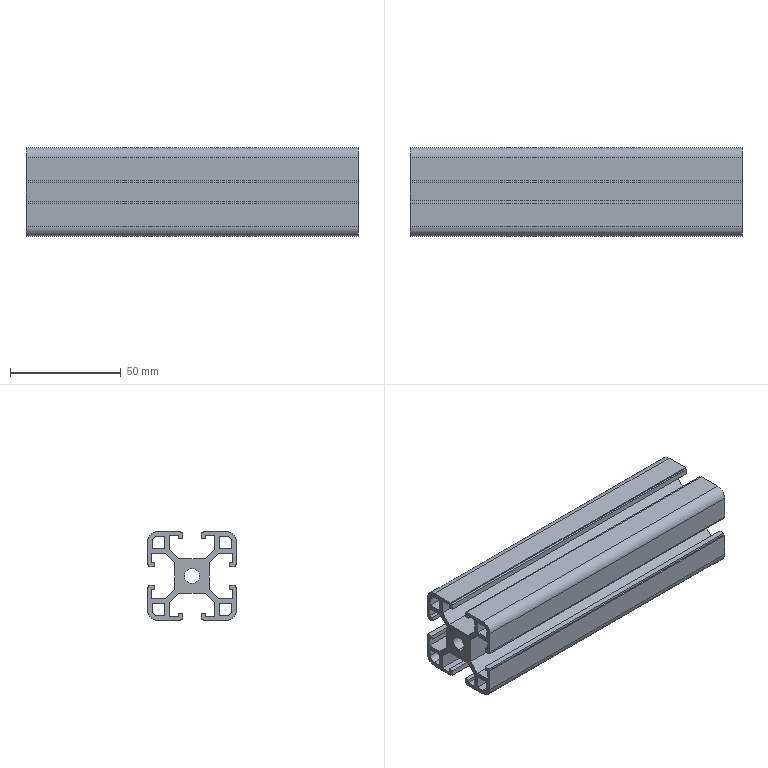Part | SolidWorks | features WeldMemberFeat 1, WeldmentFeature 1 | 1 solid | 104 faces | box 150 x 40 x 40 mm | volume 86482 mm3 | plane 94 | cylinder 10 | commonest cylinder face diameters 5 x4 9 x4 6.8 x2